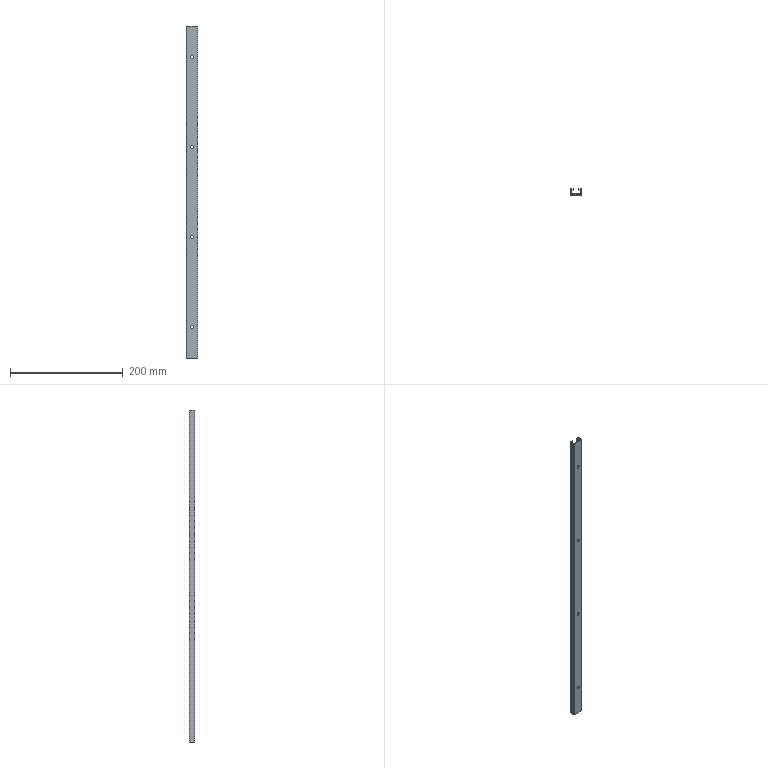Part | STEP file | 0228_Z_LGTS40-590-K4-P1602 | 1 solid | 30 faces | box 20 x 10 x 590 mm | volume 38370 mm3 | plane 22 | cylinder 8 | commonest cylinder face diameters 5.2 x8